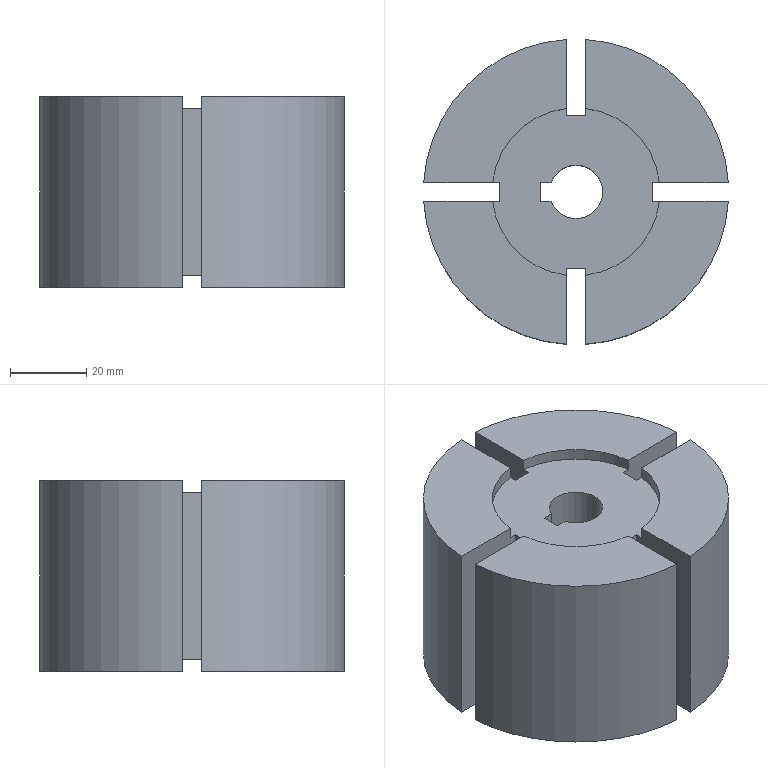Part | NX | features DATUM_CSYS 7, EXTRUDE 7, SKETCH 6, EXTRACT_DATUM_AXIS 4, EXTRACT_FACE 4, Instance Feature 3, Pattern Feature 1 | 1 solid | 38 faces | box 79.844 x 79.844 x 50 mm | volume 215152 mm3 | plane 25 | cylinder 13 | commonest cylinder face diameters 44 x8 80 x4 14 x1
STEP:
#1=CARTESIAN_POINT('',(21.857,2.5,3.));
#2=VERTEX_POINT('',#1);
#3=CARTESIAN_POINT('',(21.857,2.5,0.));
#4=VERTEX_POINT('',#3);
#5=CARTESIAN_POINT('',(21.857,2.5,50.));
#6=DIRECTION('',(0.,0.,-1.));
#7=VECTOR('',#6,1000.);
#8=LINE('',#5,#7);
#9=EDGE_CURVE('',#2,#4,#8,.T.);
#10=ORIENTED_EDGE('',*,*,#9,.F.);
#11=CARTESIAN_POINT('',(2.5,21.857,3.));
#12=VERTEX_POINT('',#11);
#13=CARTESIAN_POINT('',(0.,0.,3.));
#14=DIRECTION('',(0.,0.,1.));
#15=DIRECTION('',(1.,0.,0.));
#16=AXIS2_PLACEMENT_3D('',#13,#14,#15);
#17=CIRCLE('',#16,22.);
#18=EDGE_CURVE('',#2,#12,#17,.T.);
#19=ORIENTED_EDGE('',*,*,#18,.T.);
#20=CARTESIAN_POINT('',(2.5,21.857,0.));
#21=VERTEX_POINT('',#20);
#22=CARTESIAN_POINT('',(2.5,21.857,50.));
#23=DIRECTION('',(0.,0.,-1.));
#24=VECTOR('',#23,1000.);
#25=LINE('',#22,#24);
#26=EDGE_CURVE('',#21,#12,#25,.F.);
#27=ORIENTED_EDGE('',*,*,#26,.F.);
#28=CARTESIAN_POINT('',(0.,0.,0.));
#29=DIRECTION('',(0.,0.,1.));
#30=DIRECTION('',(1.,0.,0.));
#31=AXIS2_PLACEMENT_3D('',#28,#29,#30);
#32=CIRCLE('',#31,22.);
#33=EDGE_CURVE('',#4,#21,#32,.T.);
#34=ORIENTED_EDGE('',*,*,#33,.F.);
#35=EDGE_LOOP('',(#10,#19,#27,#34));
#36=FACE_BOUND('',#35,.T.);
#37=CARTESIAN_POINT('',(0.,0.,50.));
#38=DIRECTION('',(0.,0.,-1.));
#39=DIRECTION('',(-1.,0.,0.));
#40=AXIS2_PLACEMENT_3D('',#37,#38,#39);
#41=CYLINDRICAL_SURFACE('',#40,22.);
#42=ADVANCED_FACE('',(#36),#41,.F.);
#43=CARTESIAN_POINT('',(39.922,2.5,50.));
#44=VERTEX_POINT('',#43);
#45=CARTESIAN_POINT('',(2.5,39.922,50.));
#46=VERTEX_POINT('',#45);
#47=CARTESIAN_POINT('',(0.,0.,50.));
#48=DIRECTION('',(0.,0.,1.));
#49=DIRECTION('',(1.,0.,0.));
#50=AXIS2_PLACEMENT_3D('',#47,#48,#49);
#51=CIRCLE('',#50,40.);
#52=EDGE_CURVE('',#44,#46,#51,.T.);
#53=ORIENTED_EDGE('',*,*,#52,.F.);
#54=CARTESIAN_POINT('',(39.922,2.5,0.));
#55=VERTEX_POINT('',#54);
#56=CARTESIAN_POINT('',(39.922,2.5,50.));
#57=DIRECTION('',(0.,0.,-1.));
#58=VECTOR('',#57,1000.);
#59=LINE('',#56,#58);
#60=EDGE_CURVE('',#44,#55,#59,.T.);
#61=ORIENTED_EDGE('',*,*,#60,.T.);
#62=CARTESIAN_POINT('',(2.5,39.922,0.));
#63=VERTEX_POINT('',#62);
#64=CARTESIAN_POINT('',(0.,0.,0.));
#65=DIRECTION('',(0.,0.,1.));
#66=DIRECTION('',(1.,0.,0.));
#67=AXIS2_PLACEMENT_3D('',#64,#65,#66);
#68=CIRCLE('',#67,40.);
#69=EDGE_CURVE('',#55,#63,#68,.T.);
#70=ORIENTED_EDGE('',*,*,#69,.T.);
#71=CARTESIAN_POINT('',(2.5,39.922,50.));
#72=DIRECTION('',(0.,0.,-1.));
#73=VECTOR('',#72,1000.);
#74=LINE('',#71,#73);
#75=EDGE_CURVE('',#63,#46,#74,.F.);
#76=ORIENTED_EDGE('',*,*,#75,.T.);
#77=EDGE_LOOP('',(#53,#61,#70,#76));
#78=FACE_BOUND('',#77,.T.);
#79=CARTESIAN_POINT('',(0.,0.,50.));
#80=DIRECTION('',(0.,0.,-1.));
#81=DIRECTION('',(-1.,0.,0.));
#82=AXIS2_PLACEMENT_3D('',#79,#80,#81);
#83=CYLINDRICAL_SURFACE('',#82,40.);
#84=ADVANCED_FACE('',(#78),#83,.T.);
#85=CARTESIAN_POINT('',(21.857,2.5,50.));
#86=VERTEX_POINT('',#85);
#87=CARTESIAN_POINT('',(21.857,2.5,47.));
#88=VERTEX_POINT('',#87);
#89=CARTESIAN_POINT('',(21.857,2.5,50.));
#90=DIRECTION('',(0.,0.,-1.));
#91=VECTOR('',#90,1000.);
#92=LINE('',#89,#91);
#93=EDGE_CURVE('',#86,#88,#92,.T.);
#94=ORIENTED_EDGE('',*,*,#93,.F.);
#95=CARTESIAN_POINT('',(2.5,21.857,50.));
#96=VERTEX_POINT('',#95);
#97=CARTESIAN_POINT('',(0.,0.,50.));
#98=DIRECTION('',(0.,0.,1.));
#99=DIRECTION('',(1.,0.,0.));
#100=AXIS2_PLACEMENT_3D('',#97,#98,#99);
#101=CIRCLE('',#100,22.);
#102=EDGE_CURVE('',#86,#96,#101,.T.);
#103=ORIENTED_EDGE('',*,*,#102,.T.);
#104=CARTESIAN_POINT('',(2.5,21.857,47.));
#105=VERTEX_POINT('',#104);
#106=CARTESIAN_POINT('',(2.5,21.857,50.));
#107=DIRECTION('',(0.,0.,-1.));
#108=VECTOR('',#107,1000.);
#109=LINE('',#106,#108);
#110=EDGE_CURVE('',#105,#96,#109,.F.);
#111=ORIENTED_EDGE('',*,*,#110,.F.);
#112=CARTESIAN_POINT('',(0.,0.,47.));
#113=DIRECTION('',(0.,0.,1.));
#114=DIRECTION('',(1.,0.,0.));
#115=AXIS2_PLACEMENT_3D('',#112,#113,#114);
#116=CIRCLE('',#115,22.);
#117=EDGE_CURVE('',#88,#105,#116,.T.);
#118=ORIENTED_EDGE('',*,*,#117,.F.);
#119=EDGE_LOOP('',(#94,#103,#111,#118));
#120=FACE_BOUND('',#119,.T.);
#121=CARTESIAN_POINT('',(0.,0.,50.));
#122=DIRECTION('',(0.,0.,-1.));
#123=DIRECTION('',(-1.,0.,0.));
#124=AXIS2_PLACEMENT_3D('',#121,#122,#123);
#125=CYLINDRICAL_SURFACE('',#124,22.);
#126=ADVANCED_FACE('',(#120),#125,.F.);
#127=CARTESIAN_POINT('',(49.912,2.5,50.));
#128=DIRECTION('',(-1.,0.,0.));
#129=VECTOR('',#128,1000.);
#130=LINE('',#127,#129);
#131=EDGE_CURVE('',#44,#86,#130,.T.);
#132=ORIENTED_EDGE('',*,*,#131,.F.);
#133=ORIENTED_EDGE('',*,*,#52,.T.);
#134=CARTESIAN_POINT('',(2.5,20.,50.));
#135=DIRECTION('',(0.,1.,0.));
#136=VECTOR('',#135,1000.);
#137=LINE('',#134,#136);
#138=EDGE_CURVE('',#96,#46,#137,.T.);
#139=ORIENTED_EDGE('',*,*,#138,.F.);
#140=ORIENTED_EDGE('',*,*,#102,.F.);
#141=EDGE_LOOP('',(#132,#133,#139,#140));
#142=FACE_BOUND('',#141,.T.);
#143=CARTESIAN_POINT('',(0.,0.,50.));
#144=DIRECTION('',(0.,0.,1.));
#145=DIRECTION('',(1.,0.,0.));
#146=AXIS2_PLACEMENT_3D('',#143,#144,#145);
#147=PLANE('',#146);
#148=ADVANCED_FACE('',(#142),#147,.T.);
#149=ORIENTED_EDGE('',*,*,#69,.F.);
#150=CARTESIAN_POINT('',(49.912,2.5,0.));
#151=DIRECTION('',(-1.,0.,0.));
#152=VECTOR('',#151,1000.);
#153=LINE('',#150,#152);
#154=EDGE_CURVE('',#55,#4,#153,.T.);
#155=ORIENTED_EDGE('',*,*,#154,.T.);
#156=ORIENTED_EDGE('',*,*,#33,.T.);
#157=CARTESIAN_POINT('',(2.5,20.,0.));
#158=DIRECTION('',(0.,1.,0.));
#159=VECTOR('',#158,1000.);
#160=LINE('',#157,#159);
#161=EDGE_CURVE('',#21,#63,#160,.T.);
#162=ORIENTED_EDGE('',*,*,#161,.T.);
#163=EDGE_LOOP('',(#149,#155,#156,#162));
#164=FACE_BOUND('',#163,.T.);
#165=CARTESIAN_POINT('',(0.,0.,0.));
#166=DIRECTION('',(0.,0.,1.));
#167=DIRECTION('',(1.,0.,0.));
#168=AXIS2_PLACEMENT_3D('',#165,#166,#167);
#169=PLANE('',#168);
#170=ADVANCED_FACE('',(#164),#169,.F.);
#171=CARTESIAN_POINT('',(21.857,-2.5,0.));
#172=VERTEX_POINT('',#171);
#173=CARTESIAN_POINT('',(21.857,-2.5,3.));
#174=VERTEX_POINT('',#173);
#175=CARTESIAN_POINT('',(21.857,-2.5,50.));
#176=DIRECTION('',(0.,0.,-1.));
#177=VECTOR('',#176,1000.);
#178=LINE('',#175,#177);
#179=EDGE_CURVE('',#172,#174,#178,.F.);
#180=ORIENTED_EDGE('',*,*,#179,.F.);
#181=CARTESIAN_POINT('',(2.5,-21.857,0.));
#182=VERTEX_POINT('',#181);
#183=CARTESIAN_POINT('',(0.,0.,0.));
#184=DIRECTION('',(0.,0.,1.));
#185=DIRECTION('',(1.,0.,0.));
#186=AXIS2_PLACEMENT_3D('',#183,#184,#185);
#187=CIRCLE('',#186,22.);
#188=EDGE_CURVE('',#182,#172,#187,.T.);
#189=ORIENTED_EDGE('',*,*,#188,.F.);
#190=CARTESIAN_POINT('',(2.5,-21.857,3.));
#191=VERTEX_POINT('',#190);
#192=CARTESIAN_POINT('',(2.5,-21.857,50.));
#193=DIRECTION('',(0.,0.,-1.));
#194=VECTOR('',#193,1000.);
#195=LINE('',#192,#194);
#196=EDGE_CURVE('',#191,#182,#195,.T.);
#197=ORIENTED_EDGE('',*,*,#196,.F.);
#198=CARTESIAN_POINT('',(0.,0.,3.));
#199=DIRECTION('',(0.,0.,1.));
#200=DIRECTION('',(1.,0.,0.));
#201=AXIS2_PLACEMENT_3D('',#198,#199,#200);
#202=CIRCLE('',#201,22.);
#203=EDGE_CURVE('',#191,#174,#202,.T.);
#204=ORIENTED_EDGE('',*,*,#203,.T.);
#205=EDGE_LOOP('',(#180,#189,#197,#204));
#206=FACE_BOUND('',#205,.T.);
#207=CARTESIAN_POINT('',(0.,0.,50.));
#208=DIRECTION('',(0.,0.,-1.));
#209=DIRECTION('',(-1.,0.,0.));
#210=AXIS2_PLACEMENT_3D('',#207,#208,#209);
#211=CYLINDRICAL_SURFACE('',#210,22.);
#212=ADVANCED_FACE('',(#206),#211,.F.);
#213=CARTESIAN_POINT('',(2.5,-39.922,0.));
#214=VERTEX_POINT('',#213);
#215=CARTESIAN_POINT('',(39.922,-2.5,0.));
#216=VERTEX_POINT('',#215);
#217=CARTESIAN_POINT('',(0.,0.,0.));
#218=DIRECTION('',(0.,0.,1.));
#219=DIRECTION('',(1.,0.,0.));
#220=AXIS2_PLACEMENT_3D('',#217,#218,#219);
#221=CIRCLE('',#220,40.);
#222=EDGE_CURVE('',#214,#216,#221,.T.);
#223=ORIENTED_EDGE('',*,*,#222,.T.);
#224=CARTESIAN_POINT('',(39.922,-2.5,50.));
#225=VERTEX_POINT('',#224);
#226=CARTESIAN_POINT('',(39.922,-2.5,50.));
#227=DIRECTION('',(0.,0.,-1.));
#228=VECTOR('',#227,1000.);
#229=LINE('',#226,#228);
#230=EDGE_CURVE('',#216,#225,#229,.F.);
#231=ORIENTED_EDGE('',*,*,#230,.T.);
#232=CARTESIAN_POINT('',(2.5,-39.922,50.));
#233=VERTEX_POINT('',#232);
#234=CARTESIAN_POINT('',(0.,0.,50.));
#235=DIRECTION('',(0.,0.,1.));
#236=DIRECTION('',(1.,0.,0.));
#237=AXIS2_PLACEMENT_3D('',#234,#235,#236);
#238=CIRCLE('',#237,40.);
#239=EDGE_CURVE('',#233,#225,#238,.T.);
#240=ORIENTED_EDGE('',*,*,#239,.F.);
#241=CARTESIAN_POINT('',(2.5,-39.922,50.));
#242=DIRECTION('',(0.,0.,-1.));
#243=VECTOR('',#242,1000.);
#244=LINE('',#241,#243);
#245=EDGE_CURVE('',#233,#214,#244,.T.);
#246=ORIENTED_EDGE('',*,*,#245,.T.);
#247=EDGE_LOOP('',(#223,#231,#240,#246));
#248=FACE_BOUND('',#247,.T.);
#249=CARTESIAN_POINT('',(0.,0.,50.));
#250=DIRECTION('',(0.,0.,-1.));
#251=DIRECTION('',(-1.,0.,0.));
#252=AXIS2_PLACEMENT_3D('',#249,#250,#251);
#253=CYLINDRICAL_SURFACE('',#252,40.);
#254=ADVANCED_FACE('',(#248),#253,.T.);
#255=CARTESIAN_POINT('',(21.857,-2.5,47.));
#256=VERTEX_POINT('',#255);
#257=CARTESIAN_POINT('',(21.857,-2.5,50.));
#258=VERTEX_POINT('',#257);
#259=CARTESIAN_POINT('',(21.857,-2.5,50.));
#260=DIRECTION('',(0.,0.,-1.));
#261=VECTOR('',#260,1000.);
#262=LINE('',#259,#261);
#263=EDGE_CURVE('',#256,#258,#262,.F.);
#264=ORIENTED_EDGE('',*,*,#263,.F.);
#265=CARTESIAN_POINT('',(2.5,-21.857,47.));
#266=VERTEX_POINT('',#265);
#267=CARTESIAN_POINT('',(0.,0.,47.));
#268=DIRECTION('',(0.,0.,1.));
#269=DIRECTION('',(1.,0.,0.));
#270=AXIS2_PLACEMENT_3D('',#267,#268,#269);
#271=CIRCLE('',#270,22.);
#272=EDGE_CURVE('',#266,#256,#271,.T.);
#273=ORIENTED_EDGE('',*,*,#272,.F.);
#274=CARTESIAN_POINT('',(2.5,-21.857,50.));
#275=VERTEX_POINT('',#274);
#276=CARTESIAN_POINT('',(2.5,-21.857,50.));
#277=DIRECTION('',(0.,0.,-1.));
#278=VECTOR('',#277,1000.);
#279=LINE('',#276,#278);
#280=EDGE_CURVE('',#275,#266,#279,.T.);
#281=ORIENTED_EDGE('',*,*,#280,.F.);
#282=CARTESIAN_POINT('',(0.,0.,50.));
#283=DIRECTION('',(0.,0.,1.));
#284=DIRECTION('',(1.,0.,0.));
#285=AXIS2_PLACEMENT_3D('',#282,#283,#284);
#286=CIRCLE('',#285,22.);
#287=EDGE_CURVE('',#275,#258,#286,.T.);
#288=ORIENTED_EDGE('',*,*,#287,.T.);
#289=EDGE_LOOP('',(#264,#273,#281,#288));
#290=FACE_BOUND('',#289,.T.);
#291=CARTESIAN_POINT('',(0.,0.,50.));
#292=DIRECTION('',(0.,0.,-1.));
#293=DIRECTION('',(-1.,0.,0.));
#294=AXIS2_PLACEMENT_3D('',#291,#292,#293);
#295=CYLINDRICAL_SURFACE('',#294,22.);
#296=ADVANCED_FACE('',(#290),#295,.F.);
#297=CARTESIAN_POINT('',(20.,-2.5,50.));
#298=DIRECTION('',(1.,0.,0.));
#299=VECTOR('',#298,1000.);
#300=LINE('',#297,#299);
#301=EDGE_CURVE('',#258,#225,#300,.T.);
#302=ORIENTED_EDGE('',*,*,#301,.F.);
#303=ORIENTED_EDGE('',*,*,#287,.F.);
#304=CARTESIAN_POINT('',(2.5,-49.912,50.));
#305=DIRECTION('',(0.,1.,0.));
#306=VECTOR('',#305,1000.);
#307=LINE('',#304,#306);
#308=EDGE_CURVE('',#233,#275,#307,.T.);
#309=ORIENTED_EDGE('',*,*,#308,.F.);
#310=ORIENTED_EDGE('',*,*,#239,.T.);
#311=EDGE_LOOP('',(#302,#303,#309,#310));
#312=FACE_BOUND('',#311,.T.);
#313=CARTESIAN_POINT('',(0.,0.,50.));
#314=DIRECTION('',(0.,0.,1.));
#315=DIRECTION('',(1.,0.,0.));
#316=AXIS2_PLACEMENT_3D('',#313,#314,#315);
#317=PLANE('',#316);
#318=ADVANCED_FACE('',(#312),#317,.T.);
#319=ORIENTED_EDGE('',*,*,#188,.T.);
#320=CARTESIAN_POINT('',(20.,-2.5,0.));
#321=DIRECTION('',(1.,0.,0.));
#322=VECTOR('',#321,1000.);
#323=LINE('',#320,#322);
#324=EDGE_CURVE('',#172,#216,#323,.T.);
#325=ORIENTED_EDGE('',*,*,#324,.T.);
#326=ORIENTED_EDGE('',*,*,#222,.F.);
#327=CARTESIAN_POINT('',(2.5,-49.912,0.));
#328=DIRECTION('',(0.,1.,0.));
#329=VECTOR('',#328,1000.);
#330=LINE('',#327,#329);
#331=EDGE_CURVE('',#214,#182,#330,.T.);
#332=ORIENTED_EDGE('',*,*,#331,.T.);
#333=EDGE_LOOP('',(#319,#325,#326,#332));
#334=FACE_BOUND('',#333,.T.);
#335=CARTESIAN_POINT('',(0.,0.,0.));
#336=DIRECTION('',(0.,0.,1.));
#337=DIRECTION('',(1.,0.,0.));
#338=AXIS2_PLACEMENT_3D('',#335,#336,#337);
#339=PLANE('',#338);
#340=ADVANCED_FACE('',(#334),#339,.F.);
#341=CARTESIAN_POINT('',(-2.5,-21.857,0.));
#342=VERTEX_POINT('',#341);
#343=CARTESIAN_POINT('',(-2.5,-21.857,3.));
#344=VERTEX_POINT('',#343);
#345=CARTESIAN_POINT('',(-2.5,-21.857,50.));
#346=DIRECTION('',(0.,0.,-1.));
#347=VECTOR('',#346,1000.);
#348=LINE('',#345,#347);
#349=EDGE_CURVE('',#342,#344,#348,.F.);
#350=ORIENTED_EDGE('',*,*,#349,.F.);
#351=CARTESIAN_POINT('',(-21.857,-2.5,0.));
#352=VERTEX_POINT('',#351);
#353=CARTESIAN_POINT('',(0.,0.,0.));
#354=DIRECTION('',(0.,0.,1.));
#355=DIRECTION('',(1.,0.,0.));
#356=AXIS2_PLACEMENT_3D('',#353,#354,#355);
#357=CIRCLE('',#356,22.);
#358=EDGE_CURVE('',#352,#342,#357,.T.);
#359=ORIENTED_EDGE('',*,*,#358,.F.);
#360=CARTESIAN_POINT('',(-21.857,-2.5,3.));
#361=VERTEX_POINT('',#360);
#362=CARTESIAN_POINT('',(-21.857,-2.5,50.));
#363=DIRECTION('',(0.,0.,-1.));
#364=VECTOR('',#363,1000.);
#365=LINE('',#362,#364);
#366=EDGE_CURVE('',#361,#352,#365,.T.);
#367=ORIENTED_EDGE('',*,*,#366,.F.);
#368=CARTESIAN_POINT('',(0.,0.,3.));
#369=DIRECTION('',(0.,0.,1.));
#370=DIRECTION('',(1.,0.,0.));
#371=AXIS2_PLACEMENT_3D('',#368,#369,#370);
#372=CIRCLE('',#371,22.);
#373=EDGE_CURVE('',#361,#344,#372,.T.);
#374=ORIENTED_EDGE('',*,*,#373,.T.);
#375=EDGE_LOOP('',(#350,#359,#367,#374));
#376=FACE_BOUND('',#375,.T.);
#377=CARTESIAN_POINT('',(0.,0.,50.));
#378=DIRECTION('',(0.,0.,-1.));
#379=DIRECTION('',(-1.,0.,0.));
#380=AXIS2_PLACEMENT_3D('',#377,#378,#379);
#381=CYLINDRICAL_SURFACE('',#380,22.);
#382=ADVANCED_FACE('',(#376),#381,.F.);
#383=CARTESIAN_POINT('',(-39.922,-2.5,0.));
#384=VERTEX_POINT('',#383);
#385=CARTESIAN_POINT('',(-2.5,-39.922,0.));
#386=VERTEX_POINT('',#385);
#387=CARTESIAN_POINT('',(0.,0.,0.));
#388=DIRECTION('',(0.,0.,1.));
#389=DIRECTION('',(1.,0.,0.));
#390=AXIS2_PLACEMENT_3D('',#387,#388,#389);
#391=CIRCLE('',#390,40.);
#392=EDGE_CURVE('',#384,#386,#391,.T.);
#393=ORIENTED_EDGE('',*,*,#392,.T.);
#394=CARTESIAN_POINT('',(-2.5,-39.922,50.));
#395=VERTEX_POINT('',#394);
#396=CARTESIAN_POINT('',(-2.5,-39.922,50.));
#397=DIRECTION('',(0.,0.,-1.));
#398=VECTOR('',#397,1000.);
#399=LINE('',#396,#398);
#400=EDGE_CURVE('',#386,#395,#399,.F.);
#401=ORIENTED_EDGE('',*,*,#400,.T.);
#402=CARTESIAN_POINT('',(-39.922,-2.5,50.));
#403=VERTEX_POINT('',#402);
#404=CARTESIAN_POINT('',(0.,0.,50.));
#405=DIRECTION('',(0.,0.,1.));
#406=DIRECTION('',(1.,0.,0.));
#407=AXIS2_PLACEMENT_3D('',#404,#405,#406);
#408=CIRCLE('',#407,40.);
#409=EDGE_CURVE('',#403,#395,#408,.T.);
#410=ORIENTED_EDGE('',*,*,#409,.F.);
#411=CARTESIAN_POINT('',(-39.922,-2.5,50.));
#412=DIRECTION('',(0.,0.,-1.));
#413=VECTOR('',#412,1000.);
#414=LINE('',#411,#413);
#415=EDGE_CURVE('',#403,#384,#414,.T.);
#416=ORIENTED_EDGE('',*,*,#415,.T.);
#417=EDGE_LOOP('',(#393,#401,#410,#416));
#418=FACE_BOUND('',#417,.T.);
#419=CARTESIAN_POINT('',(0.,0.,50.));
#420=DIRECTION('',(0.,0.,-1.));
#421=DIRECTION('',(-1.,0.,0.));
#422=AXIS2_PLACEMENT_3D('',#419,#420,#421);
#423=CYLINDRICAL_SURFACE('',#422,40.);
#424=ADVANCED_FACE('',(#418),#423,.T.);
#425=CARTESIAN_POINT('',(-2.5,-21.857,47.));
#426=VERTEX_POINT('',#425);
#427=CARTESIAN_POINT('',(-2.5,-21.857,50.));
#428=VERTEX_POINT('',#427);
#429=CARTESIAN_POINT('',(-2.5,-21.857,50.));
#430=DIRECTION('',(0.,0.,-1.));
#431=VECTOR('',#430,1000.);
#432=LINE('',#429,#431);
#433=EDGE_CURVE('',#426,#428,#432,.F.);
#434=ORIENTED_EDGE('',*,*,#433,.F.);
#435=CARTESIAN_POINT('',(-21.857,-2.5,47.));
#436=VERTEX_POINT('',#435);
#437=CARTESIAN_POINT('',(0.,0.,47.));
#438=DIRECTION('',(0.,0.,1.));
#439=DIRECTION('',(1.,0.,0.));
#440=AXIS2_PLACEMENT_3D('',#437,#438,#439);
#441=CIRCLE('',#440,22.);
#442=EDGE_CURVE('',#436,#426,#441,.T.);
#443=ORIENTED_EDGE('',*,*,#442,.F.);
#444=CARTESIAN_POINT('',(-21.857,-2.5,50.));
#445=VERTEX_POINT('',#444);
#446=CARTESIAN_POINT('',(-21.857,-2.5,50.));
#447=DIRECTION('',(0.,0.,-1.));
#448=VECTOR('',#447,1000.);
#449=LINE('',#446,#448);
#450=EDGE_CURVE('',#445,#436,#449,.T.);
#451=ORIENTED_EDGE('',*,*,#450,.F.);
#452=CARTESIAN_POINT('',(0.,0.,50.));
#453=DIRECTION('',(0.,0.,1.));
#454=DIRECTION('',(1.,0.,0.));
#455=AXIS2_PLACEMENT_3D('',#452,#453,#454);
#456=CIRCLE('',#455,22.);
#457=EDGE_CURVE('',#445,#428,#456,.T.);
#458=ORIENTED_EDGE('',*,*,#457,.T.);
#459=EDGE_LOOP('',(#434,#443,#451,#458));
#460=FACE_BOUND('',#459,.T.);
#461=CARTESIAN_POINT('',(0.,0.,50.));
#462=DIRECTION('',(0.,0.,-1.));
#463=DIRECTION('',(-1.,0.,0.));
#464=AXIS2_PLACEMENT_3D('',#461,#462,#463);
#465=CYLINDRICAL_SURFACE('',#464,22.);
#466=ADVANCED_FACE('',(#460),#465,.F.);
#467=CARTESIAN_POINT('',(-2.5,-20.,50.));
#468=DIRECTION('',(0.,-1.,0.));
#469=VECTOR('',#468,1000.);
#470=LINE('',#467,#469);
#471=EDGE_CURVE('',#428,#395,#470,.T.);
#472=ORIENTED_EDGE('',*,*,#471,.F.);
#473=ORIENTED_EDGE('',*,*,#457,.F.);
#474=CARTESIAN_POINT('',(-49.912,-2.5,50.));
#475=DIRECTION('',(1.,0.,0.));
#476=VECTOR('',#475,1000.);
#477=LINE('',#474,#476);
#478=EDGE_CURVE('',#403,#445,#477,.T.);
#479=ORIENTED_EDGE('',*,*,#478,.F.);
#480=ORIENTED_EDGE('',*,*,#409,.T.);
#481=EDGE_LOOP('',(#472,#473,#479,#480));
#482=FACE_BOUND('',#481,.T.);
#483=CARTESIAN_POINT('',(0.,0.,50.));
#484=DIRECTION('',(0.,0.,1.));
#485=DIRECTION('',(1.,0.,0.));
#486=AXIS2_PLACEMENT_3D('',#483,#484,#485);
#487=PLANE('',#486);
#488=ADVANCED_FACE('',(#482),#487,.T.);
#489=ORIENTED_EDGE('',*,*,#358,.T.);
#490=CARTESIAN_POINT('',(-2.5,-20.,0.));
#491=DIRECTION('',(0.,-1.,0.));
#492=VECTOR('',#491,1000.);
#493=LINE('',#490,#492);
#494=EDGE_CURVE('',#342,#386,#493,.T.);
#495=ORIENTED_EDGE('',*,*,#494,.T.);
#496=ORIENTED_EDGE('',*,*,#392,.F.);
#497=CARTESIAN_POINT('',(-49.912,-2.5,0.));
#498=DIRECTION('',(1.,0.,0.));
#499=VECTOR('',#498,1000.);
#500=LINE('',#497,#499);
#501=EDGE_CURVE('',#384,#352,#500,.T.);
#502=ORIENTED_EDGE('',*,*,#501,.T.);
#503=EDGE_LOOP('',(#489,#495,#496,#502));
#504=FACE_BOUND('',#503,.T.);
#505=CARTESIAN_POINT('',(0.,0.,0.));
#506=DIRECTION('',(0.,0.,1.));
#507=DIRECTION('',(1.,0.,0.));
#508=AXIS2_PLACEMENT_3D('',#505,#506,#507);
#509=PLANE('',#508);
#510=ADVANCED_FACE('',(#504),#509,.F.);
#511=CARTESIAN_POINT('',(-21.857,2.5,0.));
#512=VERTEX_POINT('',#511);
#513=CARTESIAN_POINT('',(-21.857,2.5,3.));
#514=VERTEX_POINT('',#513);
#515=CARTESIAN_POINT('',(-21.857,2.5,50.));
#516=DIRECTION('',(0.,0.,-1.));
#517=VECTOR('',#516,1000.);
#518=LINE('',#515,#517);
#519=EDGE_CURVE('',#512,#514,#518,.F.);
#520=ORIENTED_EDGE('',*,*,#519,.F.);
#521=CARTESIAN_POINT('',(-2.5,21.857,0.));
#522=VERTEX_POINT('',#521);
#523=CARTESIAN_POINT('',(0.,0.,0.));
#524=DIRECTION('',(0.,0.,1.));
#525=DIRECTION('',(1.,0.,0.));
#526=AXIS2_PLACEMENT_3D('',#523,#524,#525);
#527=CIRCLE('',#526,22.);
#528=EDGE_CURVE('',#522,#512,#527,.T.);
#529=ORIENTED_EDGE('',*,*,#528,.F.);
#530=CARTESIAN_POINT('',(-2.5,21.857,3.));
#531=VERTEX_POINT('',#530);
#532=CARTESIAN_POINT('',(-2.5,21.857,50.));
#533=DIRECTION('',(0.,0.,-1.));
#534=VECTOR('',#533,1000.);
#535=LINE('',#532,#534);
#536=EDGE_CURVE('',#531,#522,#535,.T.);
#537=ORIENTED_EDGE('',*,*,#536,.F.);
#538=CARTESIAN_POINT('',(0.,0.,3.));
#539=DIRECTION('',(0.,0.,1.));
#540=DIRECTION('',(1.,0.,0.));
#541=AXIS2_PLACEMENT_3D('',#538,#539,#540);
#542=CIRCLE('',#541,22.);
#543=EDGE_CURVE('',#531,#514,#542,.T.);
#544=ORIENTED_EDGE('',*,*,#543,.T.);
#545=EDGE_LOOP('',(#520,#529,#537,#544));
#546=FACE_BOUND('',#545,.T.);
#547=CARTESIAN_POINT('',(0.,0.,50.));
#548=DIRECTION('',(0.,0.,-1.));
#549=DIRECTION('',(-1.,0.,0.));
#550=AXIS2_PLACEMENT_3D('',#547,#548,#549);
#551=CYLINDRICAL_SURFACE('',#550,22.);
#552=ADVANCED_FACE('',(#546),#551,.F.);
#553=CARTESIAN_POINT('',(-2.5,39.922,0.));
#554=VERTEX_POINT('',#553);
#555=CARTESIAN_POINT('',(-39.922,2.5,0.));
#556=VERTEX_POINT('',#555);
#557=CARTESIAN_POINT('',(0.,0.,0.));
#558=DIRECTION('',(0.,0.,1.));
#559=DIRECTION('',(1.,0.,0.));
#560=AXIS2_PLACEMENT_3D('',#557,#558,#559);
#561=CIRCLE('',#560,40.);
#562=EDGE_CURVE('',#554,#556,#561,.T.);
#563=ORIENTED_EDGE('',*,*,#562,.T.);
#564=CARTESIAN_POINT('',(-39.922,2.5,50.));
#565=VERTEX_POINT('',#564);
#566=CARTESIAN_POINT('',(-39.922,2.5,50.));
#567=DIRECTION('',(0.,0.,-1.));
#568=VECTOR('',#567,1000.);
#569=LINE('',#566,#568);
#570=EDGE_CURVE('',#556,#565,#569,.F.);
#571=ORIENTED_EDGE('',*,*,#570,.T.);
#572=CARTESIAN_POINT('',(-2.5,39.922,50.));
#573=VERTEX_POINT('',#572);
#574=CARTESIAN_POINT('',(0.,0.,50.));
#575=DIRECTION('',(0.,0.,1.));
#576=DIRECTION('',(1.,0.,0.));
#577=AXIS2_PLACEMENT_3D('',#574,#575,#576);
#578=CIRCLE('',#577,40.);
#579=EDGE_CURVE('',#573,#565,#578,.T.);
#580=ORIENTED_EDGE('',*,*,#579,.F.);
#581=CARTESIAN_POINT('',(-2.5,39.922,50.));
#582=DIRECTION('',(0.,0.,-1.));
#583=VECTOR('',#582,1000.);
#584=LINE('',#581,#583);
#585=EDGE_CURVE('',#573,#554,#584,.T.);
#586=ORIENTED_EDGE('',*,*,#585,.T.);
#587=EDGE_LOOP('',(#563,#571,#580,#586));
#588=FACE_BOUND('',#587,.T.);
#589=CARTESIAN_POINT('',(0.,0.,50.));
#590=DIRECTION('',(0.,0.,-1.));
#591=DIRECTION('',(-1.,0.,0.));
#592=AXIS2_PLACEMENT_3D('',#589,#590,#591);
#593=CYLINDRICAL_SURFACE('',#592,40.);
#594=ADVANCED_FACE('',(#588),#593,.T.);
#595=CARTESIAN_POINT('',(-21.857,2.5,47.));
#596=VERTEX_POINT('',#595);
#597=CARTESIAN_POINT('',(-21.857,2.5,50.));
#598=VERTEX_POINT('',#597);
#599=CARTESIAN_POINT('',(-21.857,2.5,50.));
#600=DIRECTION('',(0.,0.,-1.));
#601=VECTOR('',#600,1000.);
#602=LINE('',#599,#601);
#603=EDGE_CURVE('',#596,#598,#602,.F.);
#604=ORIENTED_EDGE('',*,*,#603,.F.);
#605=CARTESIAN_POINT('',(-2.5,21.857,47.));
#606=VERTEX_POINT('',#605);
#607=CARTESIAN_POINT('',(0.,0.,47.));
#608=DIRECTION('',(0.,0.,1.));
#609=DIRECTION('',(1.,0.,0.));
#610=AXIS2_PLACEMENT_3D('',#607,#608,#609);
#611=CIRCLE('',#610,22.);
#612=EDGE_CURVE('',#606,#596,#611,.T.);
#613=ORIENTED_EDGE('',*,*,#612,.F.);
#614=CARTESIAN_POINT('',(-2.5,21.857,50.));
#615=VERTEX_POINT('',#614);
#616=CARTESIAN_POINT('',(-2.5,21.857,50.));
#617=DIRECTION('',(0.,0.,-1.));
#618=VECTOR('',#617,1000.);
#619=LINE('',#616,#618);
#620=EDGE_CURVE('',#615,#606,#619,.T.);
#621=ORIENTED_EDGE('',*,*,#620,.F.);
#622=CARTESIAN_POINT('',(0.,0.,50.));
#623=DIRECTION('',(0.,0.,1.));
#624=DIRECTION('',(1.,0.,0.));
#625=AXIS2_PLACEMENT_3D('',#622,#623,#624);
#626=CIRCLE('',#625,22.);
#627=EDGE_CURVE('',#615,#598,#626,.T.);
#628=ORIENTED_EDGE('',*,*,#627,.T.);
#629=EDGE_LOOP('',(#604,#613,#621,#628));
#630=FACE_BOUND('',#629,.T.);
#631=CARTESIAN_POINT('',(0.,0.,50.));
#632=DIRECTION('',(0.,0.,-1.));
#633=DIRECTION('',(-1.,0.,0.));
#634=AXIS2_PLACEMENT_3D('',#631,#632,#633);
#635=CYLINDRICAL_SURFACE('',#634,22.);
#636=ADVANCED_FACE('',(#630),#635,.F.);
#637=CARTESIAN_POINT('',(-20.,2.5,50.));
#638=DIRECTION('',(-1.,0.,0.));
#639=VECTOR('',#638,1000.);
#640=LINE('',#637,#639);
#641=EDGE_CURVE('',#598,#565,#640,.T.);
#642=ORIENTED_EDGE('',*,*,#641,.F.);
#643=ORIENTED_EDGE('',*,*,#627,.F.);
#644=CARTESIAN_POINT('',(-2.5,49.912,50.));
#645=DIRECTION('',(0.,-1.,0.));
#646=VECTOR('',#645,1000.);
#647=LINE('',#644,#646);
#648=EDGE_CURVE('',#573,#615,#647,.T.);
#649=ORIENTED_EDGE('',*,*,#648,.F.);
#650=ORIENTED_EDGE('',*,*,#579,.T.);
#651=EDGE_LOOP('',(#642,#643,#649,#650));
#652=FACE_BOUND('',#651,.T.);
#653=CARTESIAN_POINT('',(0.,0.,50.));
#654=DIRECTION('',(0.,0.,1.));
#655=DIRECTION('',(1.,0.,0.));
#656=AXIS2_PLACEMENT_3D('',#653,#654,#655);
#657=PLANE('',#656);
#658=ADVANCED_FACE('',(#652),#657,.T.);
#659=ORIENTED_EDGE('',*,*,#528,.T.);
#660=CARTESIAN_POINT('',(-20.,2.5,0.));
#661=DIRECTION('',(-1.,0.,0.));
#662=VECTOR('',#661,1000.);
#663=LINE('',#660,#662);
#664=EDGE_CURVE('',#512,#556,#663,.T.);
#665=ORIENTED_EDGE('',*,*,#664,.T.);
#666=ORIENTED_EDGE('',*,*,#562,.F.);
#667=CARTESIAN_POINT('',(-2.5,49.912,0.));
#668=DIRECTION('',(0.,-1.,0.));
#669=VECTOR('',#668,1000.);
#670=LINE('',#667,#669);
#671=EDGE_CURVE('',#554,#522,#670,.T.);
#672=ORIENTED_EDGE('',*,*,#671,.T.);
#673=EDGE_LOOP('',(#659,#665,#666,#672));
#674=FACE_BOUND('',#673,.T.);
#675=CARTESIAN_POINT('',(0.,0.,0.));
#676=DIRECTION('',(0.,0.,1.));
#677=DIRECTION('',(1.,0.,0.));
#678=AXIS2_PLACEMENT_3D('',#675,#676,#677);
#679=PLANE('',#678);
#680=ADVANCED_FACE('',(#674),#679,.F.);
#681=CARTESIAN_POINT('',(-6.538,2.5,3.));
#682=VERTEX_POINT('',#681);
#683=CARTESIAN_POINT('',(-9.3,2.5,3.));
#684=VERTEX_POINT('',#683);
#685=CARTESIAN_POINT('',(0.,2.5,3.));
#686=DIRECTION('',(-1.,0.,0.));
#687=VECTOR('',#686,1000.);
#688=LINE('',#685,#687);
#689=EDGE_CURVE('',#682,#684,#688,.T.);
#690=ORIENTED_EDGE('',*,*,#689,.T.);
#691=CARTESIAN_POINT('',(-9.3,-2.5,3.));
#692=VERTEX_POINT('',#691);
#693=CARTESIAN_POINT('',(-9.3,0.,3.));
#694=DIRECTION('',(0.,-1.,0.));
#695=VECTOR('',#694,1000.);
#696=LINE('',#693,#695);
#697=EDGE_CURVE('',#684,#692,#696,.T.);
#698=ORIENTED_EDGE('',*,*,#697,.T.);
#699=CARTESIAN_POINT('',(-6.538,-2.5,3.));
#700=VERTEX_POINT('',#699);
#701=CARTESIAN_POINT('',(0.,-2.5,3.));
#702=DIRECTION('',(1.,0.,0.));
#703=VECTOR('',#702,1000.);
#704=LINE('',#701,#703);
#705=EDGE_CURVE('',#692,#700,#704,.T.);
#706=ORIENTED_EDGE('',*,*,#705,.T.);
#707=CARTESIAN_POINT('',(0.,0.,3.));
#708=DIRECTION('',(0.,0.,1.));
#709=DIRECTION('',(1.,0.,0.));
#710=AXIS2_PLACEMENT_3D('',#707,#708,#709);
#711=CIRCLE('',#710,7.);
#712=EDGE_CURVE('',#700,#682,#711,.T.);
#713=ORIENTED_EDGE('',*,*,#712,.T.);
#714=EDGE_LOOP('',(#690,#698,#706,#713));
#715=FACE_BOUND('',#714,.T.);
#716=ORIENTED_EDGE('',*,*,#18,.F.);
#717=CARTESIAN_POINT('',(20.,2.5,3.));
#718=VERTEX_POINT('',#717);
#719=CARTESIAN_POINT('',(0.,2.5,3.));
#720=DIRECTION('',(-1.,0.,0.));
#721=VECTOR('',#720,1000.);
#722=LINE('',#719,#721);
#723=EDGE_CURVE('',#2,#718,#722,.T.);
#724=ORIENTED_EDGE('',*,*,#723,.T.);
#725=CARTESIAN_POINT('',(20.,-2.5,3.));
#726=VERTEX_POINT('',#725);
#727=CARTESIAN_POINT('',(20.,0.,3.));
#728=DIRECTION('',(0.,-1.,0.));
#729=VECTOR('',#728,1000.);
#730=LINE('',#727,#729);
#731=EDGE_CURVE('',#718,#726,#730,.T.);
#732=ORIENTED_EDGE('',*,*,#731,.T.);
#733=CARTESIAN_POINT('',(0.,-2.5,3.));
#734=DIRECTION('',(1.,0.,0.));
#735=VECTOR('',#734,1000.);
#736=LINE('',#733,#735);
#737=EDGE_CURVE('',#726,#174,#736,.T.);
#738=ORIENTED_EDGE('',*,*,#737,.T.);
#739=ORIENTED_EDGE('',*,*,#203,.F.);
#740=CARTESIAN_POINT('',(2.5,-20.,3.));
#741=VERTEX_POINT('',#740);
#742=CARTESIAN_POINT('',(2.5,0.,3.));
#743=DIRECTION('',(0.,1.,0.));
#744=VECTOR('',#743,1000.);
#745=LINE('',#742,#744);
#746=EDGE_CURVE('',#191,#741,#745,.T.);
#747=ORIENTED_EDGE('',*,*,#746,.T.);
#748=CARTESIAN_POINT('',(-2.5,-20.,3.));
#749=VERTEX_POINT('',#748);
#750=CARTESIAN_POINT('',(0.,-20.,3.));
#751=DIRECTION('',(-1.,0.,0.));
#752=VECTOR('',#751,1000.);
#753=LINE('',#750,#752);
#754=EDGE_CURVE('',#741,#749,#753,.T.);
#755=ORIENTED_EDGE('',*,*,#754,.T.);
#756=CARTESIAN_POINT('',(-2.5,0.,3.));
#757=DIRECTION('',(0.,-1.,0.));
#758=VECTOR('',#757,1000.);
#759=LINE('',#756,#758);
#760=EDGE_CURVE('',#749,#344,#759,.T.);
#761=ORIENTED_EDGE('',*,*,#760,.T.);
#762=ORIENTED_EDGE('',*,*,#373,.F.);
#763=CARTESIAN_POINT('',(-20.,-2.5,3.));
#764=VERTEX_POINT('',#763);
#765=CARTESIAN_POINT('',(0.,-2.5,3.));
#766=DIRECTION('',(1.,0.,0.));
#767=VECTOR('',#766,1000.);
#768=LINE('',#765,#767);
#769=EDGE_CURVE('',#361,#764,#768,.T.);
#770=ORIENTED_EDGE('',*,*,#769,.T.);
#771=CARTESIAN_POINT('',(-20.,2.5,3.));
#772=VERTEX_POINT('',#771);
#773=CARTESIAN_POINT('',(-20.,0.,3.));
#774=DIRECTION('',(0.,1.,0.));
#775=VECTOR('',#774,1000.);
#776=LINE('',#773,#775);
#777=EDGE_CURVE('',#764,#772,#776,.T.);
#778=ORIENTED_EDGE('',*,*,#777,.T.);
#779=CARTESIAN_POINT('',(0.,2.5,3.));
#780=DIRECTION('',(-1.,0.,0.));
#781=VECTOR('',#780,1000.);
#782=LINE('',#779,#781);
#783=EDGE_CURVE('',#772,#514,#782,.T.);
#784=ORIENTED_EDGE('',*,*,#783,.T.);
#785=ORIENTED_EDGE('',*,*,#543,.F.);
#786=CARTESIAN_POINT('',(-2.5,20.,3.));
#787=VERTEX_POINT('',#786);
#788=CARTESIAN_POINT('',(-2.5,0.,3.));
#789=DIRECTION('',(0.,-1.,0.));
#790=VECTOR('',#789,1000.);
#791=LINE('',#788,#790);
#792=EDGE_CURVE('',#531,#787,#791,.T.);
#793=ORIENTED_EDGE('',*,*,#792,.T.);
#794=CARTESIAN_POINT('',(2.5,20.,3.));
#795=VERTEX_POINT('',#794);
#796=CARTESIAN_POINT('',(0.,20.,3.));
#797=DIRECTION('',(1.,0.,0.));
#798=VECTOR('',#797,1000.);
#799=LINE('',#796,#798);
#800=EDGE_CURVE('',#787,#795,#799,.T.);
#801=ORIENTED_EDGE('',*,*,#800,.T.);
#802=CARTESIAN_POINT('',(2.5,0.,3.));
#803=DIRECTION('',(0.,1.,0.));
#804=VECTOR('',#803,1000.);
#805=LINE('',#802,#804);
#806=EDGE_CURVE('',#795,#12,#805,.T.);
#807=ORIENTED_EDGE('',*,*,#806,.T.);
#808=EDGE_LOOP('',(#716,#724,#732,#738,#739,#747,#755,#761,#762,#770,#778,#784,#785,#793,#801,#807));
#809=FACE_BOUND('',#808,.T.);
#810=CARTESIAN_POINT('',(0.,0.,3.));
#811=DIRECTION('',(0.,0.,1.));
#812=DIRECTION('',(1.,0.,0.));
#813=AXIS2_PLACEMENT_3D('',#810,#811,#812);
#814=PLANE('',#813);
#815=ADVANCED_FACE('',(#715,#809),#814,.F.);
#816=CARTESIAN_POINT('',(20.,2.5,47.));
#817=VERTEX_POINT('',#816);
#818=CARTESIAN_POINT('',(0.,2.5,47.));
#819=DIRECTION('',(-1.,0.,0.));
#820=VECTOR('',#819,1000.);
#821=LINE('',#818,#820);
#822=EDGE_CURVE('',#88,#817,#821,.T.);
#823=ORIENTED_EDGE('',*,*,#822,.F.);
#824=ORIENTED_EDGE('',*,*,#117,.T.);
#825=CARTESIAN_POINT('',(2.5,20.,47.));
#826=VERTEX_POINT('',#825);
#827=CARTESIAN_POINT('',(2.5,0.,47.));
#828=DIRECTION('',(0.,1.,0.));
#829=VECTOR('',#828,1000.);
#830=LINE('',#827,#829);
#831=EDGE_CURVE('',#826,#105,#830,.T.);
#832=ORIENTED_EDGE('',*,*,#831,.F.);
#833=CARTESIAN_POINT('',(-2.5,20.,47.));
#834=VERTEX_POINT('',#833);
#835=CARTESIAN_POINT('',(0.,20.,47.));
#836=DIRECTION('',(1.,0.,0.));
#837=VECTOR('',#836,1000.);
#838=LINE('',#835,#837);
#839=EDGE_CURVE('',#834,#826,#838,.T.);
#840=ORIENTED_EDGE('',*,*,#839,.F.);
#841=CARTESIAN_POINT('',(-2.5,0.,47.));
#842=DIRECTION('',(0.,-1.,0.));
#843=VECTOR('',#842,1000.);
#844=LINE('',#841,#843);
#845=EDGE_CURVE('',#606,#834,#844,.T.);
#846=ORIENTED_EDGE('',*,*,#845,.F.);
#847=ORIENTED_EDGE('',*,*,#612,.T.);
#848=CARTESIAN_POINT('',(-20.,2.5,47.));
#849=VERTEX_POINT('',#848);
#850=CARTESIAN_POINT('',(0.,2.5,47.));
#851=DIRECTION('',(-1.,0.,0.));
#852=VECTOR('',#851,1000.);
#853=LINE('',#850,#852);
#854=EDGE_CURVE('',#849,#596,#853,.T.);
#855=ORIENTED_EDGE('',*,*,#854,.F.);
#856=CARTESIAN_POINT('',(-20.,-2.5,47.));
#857=VERTEX_POINT('',#856);
#858=CARTESIAN_POINT('',(-20.,0.,47.));
#859=DIRECTION('',(0.,1.,0.));
#860=VECTOR('',#859,1000.);
#861=LINE('',#858,#860);
#862=EDGE_CURVE('',#857,#849,#861,.T.);
#863=ORIENTED_EDGE('',*,*,#862,.F.);
#864=CARTESIAN_POINT('',(0.,-2.5,47.));
#865=DIRECTION('',(1.,0.,0.));
#866=VECTOR('',#865,1000.);
#867=LINE('',#864,#866);
#868=EDGE_CURVE('',#436,#857,#867,.T.);
#869=ORIENTED_EDGE('',*,*,#868,.F.);
#870=ORIENTED_EDGE('',*,*,#442,.T.);
#871=CARTESIAN_POINT('',(-2.5,-20.,47.));
#872=VERTEX_POINT('',#871);
#873=CARTESIAN_POINT('',(-2.5,0.,47.));
#874=DIRECTION('',(0.,-1.,0.));
#875=VECTOR('',#874,1000.);
#876=LINE('',#873,#875);
#877=EDGE_CURVE('',#872,#426,#876,.T.);
#878=ORIENTED_EDGE('',*,*,#877,.F.);
#879=CARTESIAN_POINT('',(2.5,-20.,47.));
#880=VERTEX_POINT('',#879);
#881=CARTESIAN_POINT('',(0.,-20.,47.));
#882=DIRECTION('',(-1.,0.,0.));
#883=VECTOR('',#882,1000.);
#884=LINE('',#881,#883);
#885=EDGE_CURVE('',#880,#872,#884,.T.);
#886=ORIENTED_EDGE('',*,*,#885,.F.);
#887=CARTESIAN_POINT('',(2.5,0.,47.));
#888=DIRECTION('',(0.,1.,0.));
#889=VECTOR('',#888,1000.);
#890=LINE('',#887,#889);
#891=EDGE_CURVE('',#266,#880,#890,.T.);
#892=ORIENTED_EDGE('',*,*,#891,.F.);
#893=ORIENTED_EDGE('',*,*,#272,.T.);
#894=CARTESIAN_POINT('',(20.,-2.5,47.));
#895=VERTEX_POINT('',#894);
#896=CARTESIAN_POINT('',(0.,-2.5,47.));
#897=DIRECTION('',(1.,0.,0.));
#898=VECTOR('',#897,1000.);
#899=LINE('',#896,#898);
#900=EDGE_CURVE('',#895,#256,#899,.T.);
#901=ORIENTED_EDGE('',*,*,#900,.F.);
#902=CARTESIAN_POINT('',(20.,0.,47.));
#903=DIRECTION('',(0.,-1.,0.));
#904=VECTOR('',#903,1000.);
#905=LINE('',#902,#904);
#906=EDGE_CURVE('',#817,#895,#905,.T.);
#907=ORIENTED_EDGE('',*,*,#906,.F.);
#908=EDGE_LOOP('',(#823,#824,#832,#840,#846,#847,#855,#863,#869,#870,#878,#886,#892,#893,#901,#907));
#909=FACE_BOUND('',#908,.T.);
#910=CARTESIAN_POINT('',(-9.3,2.5,47.));
#911=VERTEX_POINT('',#910);
#912=CARTESIAN_POINT('',(-9.3,-2.5,47.));
#913=VERTEX_POINT('',#912);
#914=CARTESIAN_POINT('',(-9.3,2.5,47.));
#915=DIRECTION('',(0.,-1.,0.));
#916=VECTOR('',#915,1000.);
#917=LINE('',#914,#916);
#918=EDGE_CURVE('',#911,#913,#917,.T.);
#919=ORIENTED_EDGE('',*,*,#918,.F.);
#920=CARTESIAN_POINT('',(-6.538,2.5,47.));
#921=VERTEX_POINT('',#920);
#922=CARTESIAN_POINT('',(-6.538,2.5,47.));
#923=DIRECTION('',(-1.,0.,0.));
#924=VECTOR('',#923,1000.);
#925=LINE('',#922,#924);
#926=EDGE_CURVE('',#921,#911,#925,.T.);
#927=ORIENTED_EDGE('',*,*,#926,.F.);
#928=CARTESIAN_POINT('',(-6.538,-2.5,47.));
#929=VERTEX_POINT('',#928);
#930=CARTESIAN_POINT('',(0.,0.,47.));
#931=DIRECTION('',(0.,0.,1.));
#932=DIRECTION('',(1.,0.,0.));
#933=AXIS2_PLACEMENT_3D('',#930,#931,#932);
#934=CIRCLE('',#933,7.);
#935=EDGE_CURVE('',#929,#921,#934,.T.);
#936=ORIENTED_EDGE('',*,*,#935,.F.);
#937=CARTESIAN_POINT('',(-9.3,-2.5,47.));
#938=DIRECTION('',(1.,0.,0.));
#939=VECTOR('',#938,1000.);
#940=LINE('',#937,#939);
#941=EDGE_CURVE('',#913,#929,#940,.T.);
#942=ORIENTED_EDGE('',*,*,#941,.F.);
#943=EDGE_LOOP('',(#919,#927,#936,#942));
#944=FACE_BOUND('',#943,.T.);
#945=CARTESIAN_POINT('',(0.,0.,47.));
#946=DIRECTION('',(0.,0.,1.));
#947=DIRECTION('',(1.,0.,0.));
#948=AXIS2_PLACEMENT_3D('',#945,#946,#947);
#949=PLANE('',#948);
#950=ADVANCED_FACE('',(#909,#944),#949,.T.);
#951=CARTESIAN_POINT('',(-9.3,2.5,0.));
#952=DIRECTION('',(0.,0.,1.));
#953=VECTOR('',#952,1000.);
#954=LINE('',#951,#953);
#955=EDGE_CURVE('',#911,#684,#954,.F.);
#956=ORIENTED_EDGE('',*,*,#955,.F.);
#957=ORIENTED_EDGE('',*,*,#918,.T.);
#958=CARTESIAN_POINT('',(-9.3,-2.5,0.));
#959=DIRECTION('',(0.,0.,1.));
#960=VECTOR('',#959,1000.);
#961=LINE('',#958,#960);
#962=EDGE_CURVE('',#913,#692,#961,.F.);
#963=ORIENTED_EDGE('',*,*,#962,.T.);
#964=ORIENTED_EDGE('',*,*,#697,.F.);
#965=EDGE_LOOP('',(#956,#957,#963,#964));
#966=FACE_BOUND('',#965,.T.);
#967=CARTESIAN_POINT('',(-9.3,2.5,0.));
#968=DIRECTION('',(-1.,0.,0.));
#969=DIRECTION('',(0.,0.,1.));
#970=AXIS2_PLACEMENT_3D('',#967,#968,#969);
#971=PLANE('',#970);
#972=ADVANCED_FACE('',(#966),#971,.F.);
#973=ORIENTED_EDGE('',*,*,#962,.F.);
#974=ORIENTED_EDGE('',*,*,#941,.T.);
#975=CARTESIAN_POINT('',(-6.538,-2.5,0.));
#976=DIRECTION('',(0.,0.,1.));
#977=VECTOR('',#976,1000.);
#978=LINE('',#975,#977);
#979=EDGE_CURVE('',#929,#700,#978,.F.);
#980=ORIENTED_EDGE('',*,*,#979,.T.);
#981=ORIENTED_EDGE('',*,*,#705,.F.);
#982=EDGE_LOOP('',(#973,#974,#980,#981));
#983=FACE_BOUND('',#982,.T.);
#984=CARTESIAN_POINT('',(-9.3,-2.5,0.));
#985=DIRECTION('',(0.,-1.,0.));
#986=DIRECTION('',(1.,0.,0.));
#987=AXIS2_PLACEMENT_3D('',#984,#985,#986);
#988=PLANE('',#987);
#989=ADVANCED_FACE('',(#983),#988,.F.);
#990=ORIENTED_EDGE('',*,*,#979,.F.);
#991=ORIENTED_EDGE('',*,*,#935,.T.);
#992=CARTESIAN_POINT('',(-6.538,2.5,0.));
#993=DIRECTION('',(0.,0.,1.));
#994=VECTOR('',#993,1000.);
#995=LINE('',#992,#994);
#996=EDGE_CURVE('',#921,#682,#995,.F.);
#997=ORIENTED_EDGE('',*,*,#996,.T.);
#998=ORIENTED_EDGE('',*,*,#712,.F.);
#999=EDGE_LOOP('',(#990,#991,#997,#998));
#1000=FACE_BOUND('',#999,.T.);
#1001=CARTESIAN_POINT('',(0.,0.,0.));
#1002=DIRECTION('',(0.,0.,1.));
#1003=DIRECTION('',(1.,0.,0.));
#1004=AXIS2_PLACEMENT_3D('',#1001,#1002,#1003);
#1005=CYLINDRICAL_SURFACE('',#1004,7.);
#1006=ADVANCED_FACE('',(#1000),#1005,.F.);
#1007=ORIENTED_EDGE('',*,*,#996,.F.);
#1008=ORIENTED_EDGE('',*,*,#926,.T.);
#1009=ORIENTED_EDGE('',*,*,#955,.T.);
#1010=ORIENTED_EDGE('',*,*,#689,.F.);
#1011=EDGE_LOOP('',(#1007,#1008,#1009,#1010));
#1012=FACE_BOUND('',#1011,.T.);
#1013=CARTESIAN_POINT('',(-6.538,2.5,0.));
#1014=DIRECTION('',(0.,1.,0.));
#1015=DIRECTION('',(0.,0.,1.));
#1016=AXIS2_PLACEMENT_3D('',#1013,#1014,#1015);
#1017=PLANE('',#1016);
#1018=ADVANCED_FACE('',(#1012),#1017,.F.);
#1019=ORIENTED_EDGE('',*,*,#648,.T.);
#1020=ORIENTED_EDGE('',*,*,#620,.T.);
#1021=ORIENTED_EDGE('',*,*,#845,.T.);
#1022=CARTESIAN_POINT('',(-2.5,20.,0.));
#1023=DIRECTION('',(0.,0.,1.));
#1024=VECTOR('',#1023,1000.);
#1025=LINE('',#1022,#1024);
#1026=EDGE_CURVE('',#834,#787,#1025,.F.);
#1027=ORIENTED_EDGE('',*,*,#1026,.T.);
#1028=ORIENTED_EDGE('',*,*,#792,.F.);
#1029=ORIENTED_EDGE('',*,*,#536,.T.);
#1030=ORIENTED_EDGE('',*,*,#671,.F.);
#1031=ORIENTED_EDGE('',*,*,#585,.F.);
#1032=EDGE_LOOP('',(#1019,#1020,#1021,#1027,#1028,#1029,#1030,#1031));
#1033=FACE_BOUND('',#1032,.T.);
#1034=CARTESIAN_POINT('',(-2.5,49.912,0.));
#1035=DIRECTION('',(-1.,0.,0.));
#1036=DIRECTION('',(0.,-1.,0.));
#1037=AXIS2_PLACEMENT_3D('',#1034,#1035,#1036);
#1038=PLANE('',#1037);
#1039=ADVANCED_FACE('',(#1033),#1038,.F.);
#1040=ORIENTED_EDGE('',*,*,#1026,.F.);
#1041=ORIENTED_EDGE('',*,*,#839,.T.);
#1042=CARTESIAN_POINT('',(2.5,20.,0.));
#1043=DIRECTION('',(0.,0.,1.));
#1044=VECTOR('',#1043,1000.);
#1045=LINE('',#1042,#1044);
#1046=EDGE_CURVE('',#826,#795,#1045,.F.);
#1047=ORIENTED_EDGE('',*,*,#1046,.T.);
#1048=ORIENTED_EDGE('',*,*,#800,.F.);
#1049=EDGE_LOOP('',(#1040,#1041,#1047,#1048));
#1050=FACE_BOUND('',#1049,.T.);
#1051=CARTESIAN_POINT('',(-2.5,20.,0.));
#1052=DIRECTION('',(0.,-1.,0.));
#1053=DIRECTION('',(0.,0.,-1.));
#1054=AXIS2_PLACEMENT_3D('',#1051,#1052,#1053);
#1055=PLANE('',#1054);
#1056=ADVANCED_FACE('',(#1050),#1055,.F.);
#1057=ORIENTED_EDGE('',*,*,#161,.F.);
#1058=ORIENTED_EDGE('',*,*,#26,.T.);
#1059=ORIENTED_EDGE('',*,*,#806,.F.);
#1060=ORIENTED_EDGE('',*,*,#1046,.F.);
#1061=ORIENTED_EDGE('',*,*,#831,.T.);
#1062=ORIENTED_EDGE('',*,*,#110,.T.);
#1063=ORIENTED_EDGE('',*,*,#138,.T.);
#1064=ORIENTED_EDGE('',*,*,#75,.F.);
#1065=EDGE_LOOP('',(#1057,#1058,#1059,#1060,#1061,#1062,#1063,#1064));
#1066=FACE_BOUND('',#1065,.T.);
#1067=CARTESIAN_POINT('',(2.5,20.,0.));
#1068=DIRECTION('',(1.,0.,0.));
#1069=DIRECTION('',(0.,1.,0.));
#1070=AXIS2_PLACEMENT_3D('',#1067,#1068,#1069);
#1071=PLANE('',#1070);
#1072=ADVANCED_FACE('',(#1066),#1071,.F.);
#1073=ORIENTED_EDGE('',*,*,#478,.T.);
#1074=ORIENTED_EDGE('',*,*,#450,.T.);
#1075=ORIENTED_EDGE('',*,*,#868,.T.);
#1076=CARTESIAN_POINT('',(-20.,-2.5,0.));
#1077=DIRECTION('',(0.,0.,1.));
#1078=VECTOR('',#1077,1000.);
#1079=LINE('',#1076,#1078);
#1080=EDGE_CURVE('',#857,#764,#1079,.F.);
#1081=ORIENTED_EDGE('',*,*,#1080,.T.);
#1082=ORIENTED_EDGE('',*,*,#769,.F.);
#1083=ORIENTED_EDGE('',*,*,#366,.T.);
#1084=ORIENTED_EDGE('',*,*,#501,.F.);
#1085=ORIENTED_EDGE('',*,*,#415,.F.);
#1086=EDGE_LOOP('',(#1073,#1074,#1075,#1081,#1082,#1083,#1084,#1085));
#1087=FACE_BOUND('',#1086,.T.);
#1088=CARTESIAN_POINT('',(-49.912,-2.5,0.));
#1089=DIRECTION('',(0.,-1.,0.));
#1090=DIRECTION('',(1.,0.,0.));
#1091=AXIS2_PLACEMENT_3D('',#1088,#1089,#1090);
#1092=PLANE('',#1091);
#1093=ADVANCED_FACE('',(#1087),#1092,.F.);
#1094=ORIENTED_EDGE('',*,*,#1080,.F.);
#1095=ORIENTED_EDGE('',*,*,#862,.T.);
#1096=CARTESIAN_POINT('',(-20.,2.5,0.));
#1097=DIRECTION('',(0.,0.,1.));
#1098=VECTOR('',#1097,1000.);
#1099=LINE('',#1096,#1098);
#1100=EDGE_CURVE('',#849,#772,#1099,.F.);
#1101=ORIENTED_EDGE('',*,*,#1100,.T.);
#1102=ORIENTED_EDGE('',*,*,#777,.F.);
#1103=EDGE_LOOP('',(#1094,#1095,#1101,#1102));
#1104=FACE_BOUND('',#1103,.T.);
#1105=CARTESIAN_POINT('',(-20.,-2.5,0.));
#1106=DIRECTION('',(1.,0.,0.));
#1107=DIRECTION('',(0.,1.,0.));
#1108=AXIS2_PLACEMENT_3D('',#1105,#1106,#1107);
#1109=PLANE('',#1108);
#1110=ADVANCED_FACE('',(#1104),#1109,.F.);
#1111=ORIENTED_EDGE('',*,*,#664,.F.);
#1112=ORIENTED_EDGE('',*,*,#519,.T.);
#1113=ORIENTED_EDGE('',*,*,#783,.F.);
#1114=ORIENTED_EDGE('',*,*,#1100,.F.);
#1115=ORIENTED_EDGE('',*,*,#854,.T.);
#1116=ORIENTED_EDGE('',*,*,#603,.T.);
#1117=ORIENTED_EDGE('',*,*,#641,.T.);
#1118=ORIENTED_EDGE('',*,*,#570,.F.);
#1119=EDGE_LOOP('',(#1111,#1112,#1113,#1114,#1115,#1116,#1117,#1118));
#1120=FACE_BOUND('',#1119,.T.);
#1121=CARTESIAN_POINT('',(-20.,2.5,0.));
#1122=DIRECTION('',(0.,1.,0.));
#1123=DIRECTION('',(-1.,0.,0.));
#1124=AXIS2_PLACEMENT_3D('',#1121,#1122,#1123);
#1125=PLANE('',#1124);
#1126=ADVANCED_FACE('',(#1120),#1125,.F.);
#1127=ORIENTED_EDGE('',*,*,#308,.T.);
#1128=ORIENTED_EDGE('',*,*,#280,.T.);
#1129=ORIENTED_EDGE('',*,*,#891,.T.);
#1130=CARTESIAN_POINT('',(2.5,-20.,0.));
#1131=DIRECTION('',(0.,0.,1.));
#1132=VECTOR('',#1131,1000.);
#1133=LINE('',#1130,#1132);
#1134=EDGE_CURVE('',#880,#741,#1133,.F.);
#1135=ORIENTED_EDGE('',*,*,#1134,.T.);
#1136=ORIENTED_EDGE('',*,*,#746,.F.);
#1137=ORIENTED_EDGE('',*,*,#196,.T.);
#1138=ORIENTED_EDGE('',*,*,#331,.F.);
#1139=ORIENTED_EDGE('',*,*,#245,.F.);
#1140=EDGE_LOOP('',(#1127,#1128,#1129,#1135,#1136,#1137,#1138,#1139));
#1141=FACE_BOUND('',#1140,.T.);
#1142=CARTESIAN_POINT('',(2.5,-49.912,0.));
#1143=DIRECTION('',(1.,0.,0.));
#1144=DIRECTION('',(0.,1.,0.));
#1145=AXIS2_PLACEMENT_3D('',#1142,#1143,#1144);
#1146=PLANE('',#1145);
#1147=ADVANCED_FACE('',(#1141),#1146,.F.);
#1148=ORIENTED_EDGE('',*,*,#1134,.F.);
#1149=ORIENTED_EDGE('',*,*,#885,.T.);
#1150=CARTESIAN_POINT('',(-2.5,-20.,0.));
#1151=DIRECTION('',(0.,0.,1.));
#1152=VECTOR('',#1151,1000.);
#1153=LINE('',#1150,#1152);
#1154=EDGE_CURVE('',#872,#749,#1153,.F.);
#1155=ORIENTED_EDGE('',*,*,#1154,.T.);
#1156=ORIENTED_EDGE('',*,*,#754,.F.);
#1157=EDGE_LOOP('',(#1148,#1149,#1155,#1156));
#1158=FACE_BOUND('',#1157,.T.);
#1159=CARTESIAN_POINT('',(2.5,-20.,0.));
#1160=DIRECTION('',(0.,1.,0.));
#1161=DIRECTION('',(-1.,0.,0.));
#1162=AXIS2_PLACEMENT_3D('',#1159,#1160,#1161);
#1163=PLANE('',#1162);
#1164=ADVANCED_FACE('',(#1158),#1163,.F.);
#1165=ORIENTED_EDGE('',*,*,#494,.F.);
#1166=ORIENTED_EDGE('',*,*,#349,.T.);
#1167=ORIENTED_EDGE('',*,*,#760,.F.);
#1168=ORIENTED_EDGE('',*,*,#1154,.F.);
#1169=ORIENTED_EDGE('',*,*,#877,.T.);
#1170=ORIENTED_EDGE('',*,*,#433,.T.);
#1171=ORIENTED_EDGE('',*,*,#471,.T.);
#1172=ORIENTED_EDGE('',*,*,#400,.F.);
#1173=EDGE_LOOP('',(#1165,#1166,#1167,#1168,#1169,#1170,#1171,#1172));
#1174=FACE_BOUND('',#1173,.T.);
#1175=CARTESIAN_POINT('',(-2.5,-20.,0.));
#1176=DIRECTION('',(-1.,0.,0.));
#1177=DIRECTION('',(0.,-1.,0.));
#1178=AXIS2_PLACEMENT_3D('',#1175,#1176,#1177);
#1179=PLANE('',#1178);
#1180=ADVANCED_FACE('',(#1174),#1179,.F.);
#1181=ORIENTED_EDGE('',*,*,#131,.T.);
#1182=ORIENTED_EDGE('',*,*,#93,.T.);
#1183=ORIENTED_EDGE('',*,*,#822,.T.);
#1184=CARTESIAN_POINT('',(20.,2.5,0.));
#1185=DIRECTION('',(0.,0.,1.));
#1186=VECTOR('',#1185,1000.);
#1187=LINE('',#1184,#1186);
#1188=EDGE_CURVE('',#817,#718,#1187,.F.);
#1189=ORIENTED_EDGE('',*,*,#1188,.T.);
#1190=ORIENTED_EDGE('',*,*,#723,.F.);
#1191=ORIENTED_EDGE('',*,*,#9,.T.);
#1192=ORIENTED_EDGE('',*,*,#154,.F.);
#1193=ORIENTED_EDGE('',*,*,#60,.F.);
#1194=EDGE_LOOP('',(#1181,#1182,#1183,#1189,#1190,#1191,#1192,#1193));
#1195=FACE_BOUND('',#1194,.T.);
#1196=CARTESIAN_POINT('',(49.912,2.5,0.));
#1197=DIRECTION('',(0.,1.,0.));
#1198=DIRECTION('',(-1.,0.,0.));
#1199=AXIS2_PLACEMENT_3D('',#1196,#1197,#1198);
#1200=PLANE('',#1199);
#1201=ADVANCED_FACE('',(#1195),#1200,.F.);
#1202=ORIENTED_EDGE('',*,*,#1188,.F.);
#1203=ORIENTED_EDGE('',*,*,#906,.T.);
#1204=CARTESIAN_POINT('',(20.,-2.5,0.));
#1205=DIRECTION('',(0.,0.,1.));
#1206=VECTOR('',#1205,1000.);
#1207=LINE('',#1204,#1206);
#1208=EDGE_CURVE('',#895,#726,#1207,.F.);
#1209=ORIENTED_EDGE('',*,*,#1208,.T.);
#1210=ORIENTED_EDGE('',*,*,#731,.F.);
#1211=EDGE_LOOP('',(#1202,#1203,#1209,#1210));
#1212=FACE_BOUND('',#1211,.T.);
#1213=CARTESIAN_POINT('',(20.,2.5,0.));
#1214=DIRECTION('',(-1.,0.,0.));
#1215=DIRECTION('',(0.,-1.,0.));
#1216=AXIS2_PLACEMENT_3D('',#1213,#1214,#1215);
#1217=PLANE('',#1216);
#1218=ADVANCED_FACE('',(#1212),#1217,.F.);
#1219=ORIENTED_EDGE('',*,*,#324,.F.);
#1220=ORIENTED_EDGE('',*,*,#179,.T.);
#1221=ORIENTED_EDGE('',*,*,#737,.F.);
#1222=ORIENTED_EDGE('',*,*,#1208,.F.);
#1223=ORIENTED_EDGE('',*,*,#900,.T.);
#1224=ORIENTED_EDGE('',*,*,#263,.T.);
#1225=ORIENTED_EDGE('',*,*,#301,.T.);
#1226=ORIENTED_EDGE('',*,*,#230,.F.);
#1227=EDGE_LOOP('',(#1219,#1220,#1221,#1222,#1223,#1224,#1225,#1226));
#1228=FACE_BOUND('',#1227,.T.);
#1229=CARTESIAN_POINT('',(20.,-2.5,0.));
#1230=DIRECTION('',(0.,-1.,0.));
#1231=DIRECTION('',(1.,0.,0.));
#1232=AXIS2_PLACEMENT_3D('',#1229,#1230,#1231);
#1233=PLANE('',#1232);
#1234=ADVANCED_FACE('',(#1228),#1233,.F.);
#1235=CLOSED_SHELL('',(#42,#84,#126,#148,#170,#212,#254,#296,#318,#340,#382,#424,#466,#488,#510,#552,#594,#636,#658,#680,#815,#950,#972,#989,#1006,#1018,#1039,#1056,#1072,#1093,#1110,#1126,#1147,#1164,#1180,#1201,#1218,#1234));
#1236=MANIFOLD_SOLID_BREP('',#1235);
#1237=(LENGTH_UNIT()NAMED_UNIT(*)SI_UNIT(.MILLI.,.METRE.));
#1238=UNCERTAINTY_MEASURE_WITH_UNIT(LENGTH_MEASURE(0.00001),#1237,'','');
#1239=(NAMED_UNIT(*)PLANE_ANGLE_UNIT()SI_UNIT($,.RADIAN.));
#1240=(NAMED_UNIT(*)SI_UNIT($,.STERADIAN.)SOLID_ANGLE_UNIT());
#1241=(GEOMETRIC_REPRESENTATION_CONTEXT(3)GLOBAL_UNCERTAINTY_ASSIGNED_CONTEXT((#1238))GLOBAL_UNIT_ASSIGNED_CONTEXT((#1237,#1239,#1240))REPRESENTATION_CONTEXT('',''));
#1242=ADVANCED_BREP_SHAPE_REPRESENTATION('',(#1236),#1241);